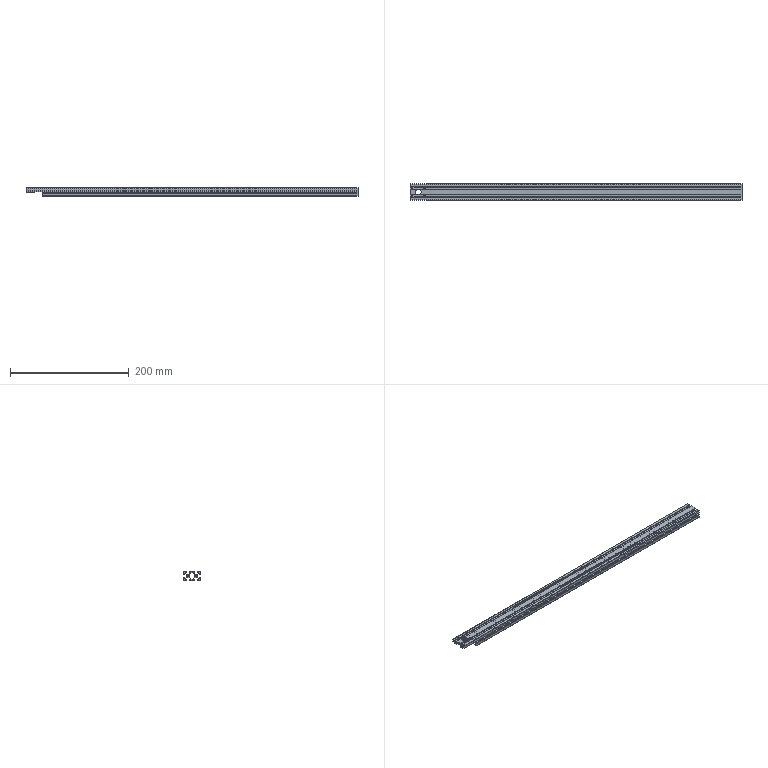Part | SolidWorks | features SplitBody 1 | 1 solid | 209 faces | box 560 x 28 x 14 mm | volume 85139 mm3 | plane 152 | cylinder 57 | commonest cylinder face diameters 0.42 x20 2.94 x16 5.6 x14 1.4 x4 9.8 x3